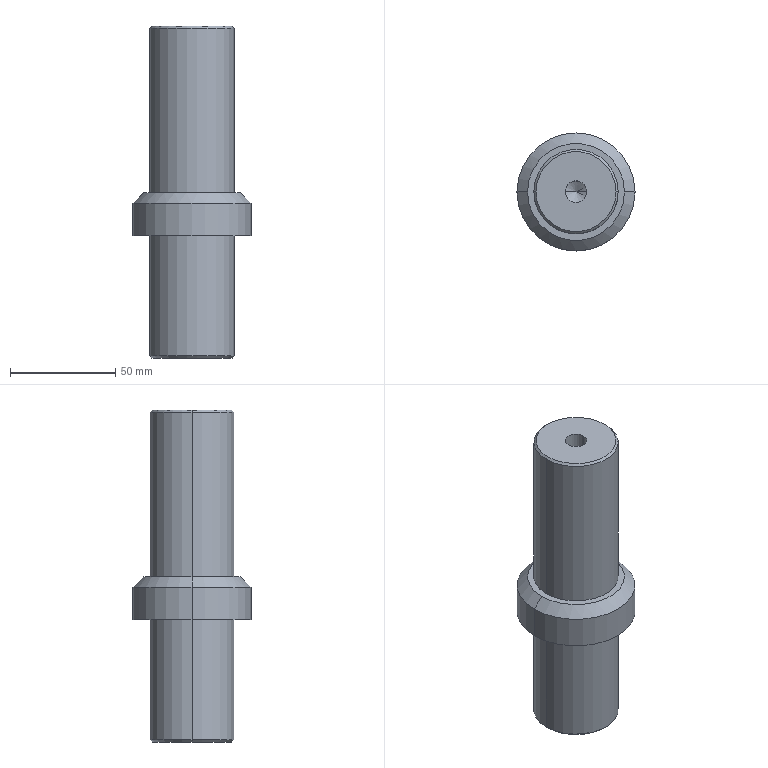Part | SolidWorks | features Chamfer 2, HoleWzd 2, ICE 2, Extrusion 1 | 1 solid | 24 faces | box 56 x 56 x 157.5 mm | volume 215391 mm3 | cylinder 10 | cone 10 | plane 4 | commonest cylinder face diameters 10.2 x4 40 x4 56 x2
STEP:
#1=CARTESIAN_POINT('',(-5.1,0.,128.25));
#2=VERTEX_POINT('',#1);
#3=CARTESIAN_POINT('',(5.1,0.,128.25));
#4=VERTEX_POINT('',#3);
#5=CARTESIAN_POINT('',(0.,0.,128.25));
#6=DIRECTION('',(0.,0.,1.));
#7=DIRECTION('',(1.,0.,0.));
#8=AXIS2_PLACEMENT_3D('',#5,#6,#7);
#9=CIRCLE('',#8,5.1);
#10=EDGE_CURVE('',#2,#4,#9,.T.);
#11=ORIENTED_EDGE('',*,*,#10,.F.);
#12=CARTESIAN_POINT('',(-5.1,0.,157.5));
#13=VERTEX_POINT('',#12);
#14=CARTESIAN_POINT('',(-5.1,0.,157.5));
#15=DIRECTION('',(0.,0.,1.));
#16=VECTOR('',#15,1000.);
#17=LINE('',#14,#16);
#18=EDGE_CURVE('',#2,#13,#17,.T.);
#19=ORIENTED_EDGE('',*,*,#18,.T.);
#20=CARTESIAN_POINT('',(5.1,0.,157.5));
#21=VERTEX_POINT('',#20);
#22=CARTESIAN_POINT('',(0.,0.,157.5));
#23=DIRECTION('',(0.,0.,1.));
#24=DIRECTION('',(1.,0.,0.));
#25=AXIS2_PLACEMENT_3D('',#22,#23,#24);
#26=CIRCLE('',#25,5.1);
#27=EDGE_CURVE('',#13,#21,#26,.T.);
#28=ORIENTED_EDGE('',*,*,#27,.T.);
#29=CARTESIAN_POINT('',(5.1,0.,157.5));
#30=DIRECTION('',(0.,0.,1.));
#31=VECTOR('',#30,1000.);
#32=LINE('',#29,#31);
#33=EDGE_CURVE('',#4,#21,#32,.T.);
#34=ORIENTED_EDGE('',*,*,#33,.F.);
#35=EDGE_LOOP('',(#11,#19,#28,#34));
#36=FACE_OUTER_BOUND('',#35,.T.);
#37=CARTESIAN_POINT('',(0.,0.,157.5));
#38=DIRECTION('',(0.,0.,1.));
#39=DIRECTION('',(1.,0.,0.));
#40=AXIS2_PLACEMENT_3D('',#37,#38,#39);
#41=CYLINDRICAL_SURFACE('',#40,5.1);
#42=ADVANCED_FACE('',(#36),#41,.F.);
#43=CARTESIAN_POINT('',(0.,0.,125.186));
#44=VERTEX_POINT('',#43);
#45=CARTESIAN_POINT('',(5.1,0.,128.25));
#46=DIRECTION('',(0.8572,0.,0.515));
#47=VECTOR('',#46,1000.);
#48=LINE('',#45,#47);
#49=EDGE_CURVE('',#44,#4,#48,.T.);
#50=ORIENTED_EDGE('',*,*,#49,.F.);
#51=CARTESIAN_POINT('',(-5.1,0.,128.25));
#52=DIRECTION('',(-0.8572,0.,0.515));
#53=VECTOR('',#52,1000.);
#54=LINE('',#51,#53);
#55=EDGE_CURVE('',#44,#2,#54,.T.);
#56=ORIENTED_EDGE('',*,*,#55,.T.);
#57=ORIENTED_EDGE('',*,*,#10,.T.);
#58=EDGE_LOOP('',(#50,#56,#57));
#59=FACE_OUTER_BOUND('',#58,.T.);
#60=CARTESIAN_POINT('',(0.,0.,128.25));
#61=DIRECTION('',(0.,0.,1.));
#62=DIRECTION('',(1.,0.,0.));
#63=AXIS2_PLACEMENT_3D('',#60,#61,#62);
#64=CONICAL_SURFACE('',#63,5.1,1.03);
#65=ADVANCED_FACE('',(#59),#64,.F.);
#66=CARTESIAN_POINT('',(5.1,0.,29.25));
#67=VERTEX_POINT('',#66);
#68=CARTESIAN_POINT('',(-5.1,0.,29.25));
#69=VERTEX_POINT('',#68);
#70=CARTESIAN_POINT('',(0.,0.,29.25));
#71=DIRECTION('',(0.,0.,-1.));
#72=DIRECTION('',(-1.,0.,0.));
#73=AXIS2_PLACEMENT_3D('',#70,#71,#72);
#74=CIRCLE('',#73,5.1);
#75=EDGE_CURVE('',#67,#69,#74,.T.);
#76=ORIENTED_EDGE('',*,*,#75,.F.);
#77=CARTESIAN_POINT('',(5.1,0.,0.));
#78=VERTEX_POINT('',#77);
#79=CARTESIAN_POINT('',(5.1,0.,0.));
#80=DIRECTION('',(0.,0.,-1.));
#81=VECTOR('',#80,1000.);
#82=LINE('',#79,#81);
#83=EDGE_CURVE('',#67,#78,#82,.T.);
#84=ORIENTED_EDGE('',*,*,#83,.T.);
#85=CARTESIAN_POINT('',(-5.1,0.,0.));
#86=VERTEX_POINT('',#85);
#87=CARTESIAN_POINT('',(0.,0.,0.));
#88=DIRECTION('',(0.,0.,-1.));
#89=DIRECTION('',(-1.,0.,0.));
#90=AXIS2_PLACEMENT_3D('',#87,#88,#89);
#91=CIRCLE('',#90,5.1);
#92=EDGE_CURVE('',#78,#86,#91,.T.);
#93=ORIENTED_EDGE('',*,*,#92,.T.);
#94=CARTESIAN_POINT('',(-5.1,0.,0.));
#95=DIRECTION('',(0.,0.,-1.));
#96=VECTOR('',#95,1000.);
#97=LINE('',#94,#96);
#98=EDGE_CURVE('',#69,#86,#97,.T.);
#99=ORIENTED_EDGE('',*,*,#98,.F.);
#100=EDGE_LOOP('',(#76,#84,#93,#99));
#101=FACE_OUTER_BOUND('',#100,.T.);
#102=CARTESIAN_POINT('',(0.,0.,0.));
#103=DIRECTION('',(0.,0.,-1.));
#104=DIRECTION('',(-1.,0.,0.));
#105=AXIS2_PLACEMENT_3D('',#102,#103,#104);
#106=CYLINDRICAL_SURFACE('',#105,5.1);
#107=ADVANCED_FACE('',(#101),#106,.F.);
#108=CARTESIAN_POINT('',(0.,0.,32.314));
#109=VERTEX_POINT('',#108);
#110=CARTESIAN_POINT('',(-5.1,0.,29.25));
#111=DIRECTION('',(-0.8572,0.,-0.515));
#112=VECTOR('',#111,1000.);
#113=LINE('',#110,#112);
#114=EDGE_CURVE('',#109,#69,#113,.T.);
#115=ORIENTED_EDGE('',*,*,#114,.F.);
#116=CARTESIAN_POINT('',(5.1,0.,29.25));
#117=DIRECTION('',(0.8572,0.,-0.515));
#118=VECTOR('',#117,1000.);
#119=LINE('',#116,#118);
#120=EDGE_CURVE('',#109,#67,#119,.T.);
#121=ORIENTED_EDGE('',*,*,#120,.T.);
#122=ORIENTED_EDGE('',*,*,#75,.T.);
#123=EDGE_LOOP('',(#115,#121,#122));
#124=FACE_OUTER_BOUND('',#123,.T.);
#125=CARTESIAN_POINT('',(0.,0.,29.25));
#126=DIRECTION('',(0.,0.,-1.));
#127=DIRECTION('',(-1.,0.,0.));
#128=AXIS2_PLACEMENT_3D('',#125,#126,#127);
#129=CONICAL_SURFACE('',#128,5.1,1.03);
#130=ADVANCED_FACE('',(#124),#129,.F.);
#131=CARTESIAN_POINT('',(-19.,0.,0.));
#132=VERTEX_POINT('',#131);
#133=CARTESIAN_POINT('',(19.,0.,0.));
#134=VERTEX_POINT('',#133);
#135=CARTESIAN_POINT('',(0.,0.,0.));
#136=DIRECTION('',(0.,0.,-1.));
#137=DIRECTION('',(1.,0.,0.));
#138=AXIS2_PLACEMENT_3D('',#135,#136,#137);
#139=CIRCLE('',#138,19.);
#140=EDGE_CURVE('',#132,#134,#139,.T.);
#141=ORIENTED_EDGE('',*,*,#140,.F.);
#142=CARTESIAN_POINT('',(-20.,0.,1.));
#143=VERTEX_POINT('',#142);
#144=CARTESIAN_POINT('',(-20.,0.,1.));
#145=DIRECTION('',(-0.7071,0.,0.7071));
#146=VECTOR('',#145,1000.);
#147=LINE('',#144,#146);
#148=EDGE_CURVE('',#132,#143,#147,.T.);
#149=ORIENTED_EDGE('',*,*,#148,.T.);
#150=CARTESIAN_POINT('',(20.,0.,1.));
#151=VERTEX_POINT('',#150);
#152=CARTESIAN_POINT('',(0.,0.,1.));
#153=DIRECTION('',(0.,0.,1.));
#154=DIRECTION('',(1.,0.,0.));
#155=AXIS2_PLACEMENT_3D('',#152,#153,#154);
#156=CIRCLE('',#155,20.);
#157=EDGE_CURVE('',#151,#143,#156,.T.);
#158=ORIENTED_EDGE('',*,*,#157,.F.);
#159=CARTESIAN_POINT('',(20.,0.,1.));
#160=DIRECTION('',(0.7071,0.,0.7071));
#161=VECTOR('',#160,1000.);
#162=LINE('',#159,#161);
#163=EDGE_CURVE('',#134,#151,#162,.T.);
#164=ORIENTED_EDGE('',*,*,#163,.F.);
#165=EDGE_LOOP('',(#141,#149,#158,#164));
#166=FACE_OUTER_BOUND('',#165,.T.);
#167=CARTESIAN_POINT('',(0.,0.,1.));
#168=DIRECTION('',(0.,0.,1.));
#169=DIRECTION('',(1.,0.,0.));
#170=AXIS2_PLACEMENT_3D('',#167,#168,#169);
#171=CONICAL_SURFACE('',#170,20.,0.7854);
#172=ADVANCED_FACE('',(#166),#171,.T.);
#173=CARTESIAN_POINT('',(19.,0.,157.5));
#174=VERTEX_POINT('',#173);
#175=CARTESIAN_POINT('',(-19.,0.,157.5));
#176=VERTEX_POINT('',#175);
#177=CARTESIAN_POINT('',(0.,0.,157.5));
#178=DIRECTION('',(0.,0.,1.));
#179=DIRECTION('',(1.,0.,0.));
#180=AXIS2_PLACEMENT_3D('',#177,#178,#179);
#181=CIRCLE('',#180,19.);
#182=EDGE_CURVE('',#174,#176,#181,.T.);
#183=ORIENTED_EDGE('',*,*,#182,.F.);
#184=CARTESIAN_POINT('',(20.,0.,156.5));
#185=VERTEX_POINT('',#184);
#186=CARTESIAN_POINT('',(19.,0.,157.5));
#187=DIRECTION('',(0.7071,0.,-0.7071));
#188=VECTOR('',#187,1000.);
#189=LINE('',#186,#188);
#190=EDGE_CURVE('',#174,#185,#189,.T.);
#191=ORIENTED_EDGE('',*,*,#190,.T.);
#192=CARTESIAN_POINT('',(-20.,0.,156.5));
#193=VERTEX_POINT('',#192);
#194=CARTESIAN_POINT('',(0.,0.,156.5));
#195=DIRECTION('',(0.,0.,-1.));
#196=DIRECTION('',(1.,0.,0.));
#197=AXIS2_PLACEMENT_3D('',#194,#195,#196);
#198=CIRCLE('',#197,20.);
#199=EDGE_CURVE('',#193,#185,#198,.T.);
#200=ORIENTED_EDGE('',*,*,#199,.F.);
#201=CARTESIAN_POINT('',(-19.,0.,157.5));
#202=DIRECTION('',(-0.7071,0.,-0.7071));
#203=VECTOR('',#202,1000.);
#204=LINE('',#201,#203);
#205=EDGE_CURVE('',#176,#193,#204,.T.);
#206=ORIENTED_EDGE('',*,*,#205,.F.);
#207=EDGE_LOOP('',(#183,#191,#200,#206));
#208=FACE_OUTER_BOUND('',#207,.T.);
#209=CARTESIAN_POINT('',(0.,0.,157.5));
#210=DIRECTION('',(0.,0.,-1.));
#211=DIRECTION('',(-1.,0.,0.));
#212=AXIS2_PLACEMENT_3D('',#209,#210,#211);
#213=CONICAL_SURFACE('',#212,19.,0.7854);
#214=ADVANCED_FACE('',(#208),#213,.T.);
#215=CARTESIAN_POINT('',(23.,0.,78.4));
#216=VERTEX_POINT('',#215);
#217=CARTESIAN_POINT('',(-23.,0.,78.4));
#218=VERTEX_POINT('',#217);
#219=CARTESIAN_POINT('',(0.,0.,78.4));
#220=DIRECTION('',(0.,0.,1.));
#221=DIRECTION('',(1.,0.,0.));
#222=AXIS2_PLACEMENT_3D('',#219,#220,#221);
#223=CIRCLE('',#222,23.);
#224=EDGE_CURVE('',#216,#218,#223,.T.);
#225=ORIENTED_EDGE('',*,*,#224,.F.);
#226=CARTESIAN_POINT('',(28.,0.,73.4));
#227=VERTEX_POINT('',#226);
#228=CARTESIAN_POINT('',(23.,0.,78.4));
#229=DIRECTION('',(0.7071,0.,-0.7071));
#230=VECTOR('',#229,1000.);
#231=LINE('',#228,#230);
#232=EDGE_CURVE('',#216,#227,#231,.T.);
#233=ORIENTED_EDGE('',*,*,#232,.T.);
#234=CARTESIAN_POINT('',(-28.,0.,73.4));
#235=VERTEX_POINT('',#234);
#236=CARTESIAN_POINT('',(0.,0.,73.4));
#237=DIRECTION('',(0.,0.,-1.));
#238=DIRECTION('',(1.,0.,0.));
#239=AXIS2_PLACEMENT_3D('',#236,#237,#238);
#240=CIRCLE('',#239,28.);
#241=EDGE_CURVE('',#235,#227,#240,.T.);
#242=ORIENTED_EDGE('',*,*,#241,.F.);
#243=CARTESIAN_POINT('',(-23.,0.,78.4));
#244=DIRECTION('',(-0.7071,0.,-0.7071));
#245=VECTOR('',#244,1000.);
#246=LINE('',#243,#245);
#247=EDGE_CURVE('',#218,#235,#246,.T.);
#248=ORIENTED_EDGE('',*,*,#247,.F.);
#249=EDGE_LOOP('',(#225,#233,#242,#248));
#250=FACE_OUTER_BOUND('',#249,.T.);
#251=CARTESIAN_POINT('',(0.,0.,78.4));
#252=DIRECTION('',(0.,0.,-1.));
#253=DIRECTION('',(-1.,0.,0.));
#254=AXIS2_PLACEMENT_3D('',#251,#252,#253);
#255=CONICAL_SURFACE('',#254,23.,0.7854);
#256=ADVANCED_FACE('',(#250),#255,.T.);
#257=ORIENTED_EDGE('',*,*,#199,.T.);
#258=CARTESIAN_POINT('',(20.,0.,78.4));
#259=VERTEX_POINT('',#258);
#260=CARTESIAN_POINT('',(20.,0.,157.5));
#261=DIRECTION('',(0.,0.,-1.));
#262=VECTOR('',#261,1000.);
#263=LINE('',#260,#262);
#264=EDGE_CURVE('',#185,#259,#263,.T.);
#265=ORIENTED_EDGE('',*,*,#264,.T.);
#266=CARTESIAN_POINT('',(-20.,0.,78.4));
#267=VERTEX_POINT('',#266);
#268=CARTESIAN_POINT('',(0.,0.,78.4));
#269=DIRECTION('',(0.,0.,1.));
#270=DIRECTION('',(1.,0.,0.));
#271=AXIS2_PLACEMENT_3D('',#268,#269,#270);
#272=CIRCLE('',#271,20.);
#273=EDGE_CURVE('',#259,#267,#272,.T.);
#274=ORIENTED_EDGE('',*,*,#273,.T.);
#275=CARTESIAN_POINT('',(-20.,0.,157.5));
#276=DIRECTION('',(0.,0.,-1.));
#277=VECTOR('',#276,1000.);
#278=LINE('',#275,#277);
#279=EDGE_CURVE('',#193,#267,#278,.T.);
#280=ORIENTED_EDGE('',*,*,#279,.F.);
#281=EDGE_LOOP('',(#257,#265,#274,#280));
#282=FACE_OUTER_BOUND('',#281,.T.);
#283=CARTESIAN_POINT('',(0.,0.,157.5));
#284=DIRECTION('',(0.,0.,-1.));
#285=DIRECTION('',(-1.,0.,0.));
#286=AXIS2_PLACEMENT_3D('',#283,#284,#285);
#287=CYLINDRICAL_SURFACE('',#286,20.);
#288=ADVANCED_FACE('',(#282),#287,.T.);
#289=ORIENTED_EDGE('',*,*,#241,.T.);
#290=CARTESIAN_POINT('',(28.,0.,58.));
#291=VERTEX_POINT('',#290);
#292=CARTESIAN_POINT('',(28.,0.,78.4));
#293=DIRECTION('',(0.,0.,-1.));
#294=VECTOR('',#293,1000.);
#295=LINE('',#292,#294);
#296=EDGE_CURVE('',#227,#291,#295,.T.);
#297=ORIENTED_EDGE('',*,*,#296,.T.);
#298=CARTESIAN_POINT('',(-28.,0.,58.));
#299=VERTEX_POINT('',#298);
#300=CARTESIAN_POINT('',(0.,0.,58.));
#301=DIRECTION('',(0.,0.,1.));
#302=DIRECTION('',(1.,0.,0.));
#303=AXIS2_PLACEMENT_3D('',#300,#301,#302);
#304=CIRCLE('',#303,28.);
#305=EDGE_CURVE('',#291,#299,#304,.T.);
#306=ORIENTED_EDGE('',*,*,#305,.T.);
#307=CARTESIAN_POINT('',(-28.,0.,78.4));
#308=DIRECTION('',(0.,0.,-1.));
#309=VECTOR('',#308,1000.);
#310=LINE('',#307,#309);
#311=EDGE_CURVE('',#235,#299,#310,.T.);
#312=ORIENTED_EDGE('',*,*,#311,.F.);
#313=EDGE_LOOP('',(#289,#297,#306,#312));
#314=FACE_OUTER_BOUND('',#313,.T.);
#315=CARTESIAN_POINT('',(0.,0.,78.4));
#316=DIRECTION('',(0.,0.,-1.));
#317=DIRECTION('',(-1.,0.,0.));
#318=AXIS2_PLACEMENT_3D('',#315,#316,#317);
#319=CYLINDRICAL_SURFACE('',#318,28.);
#320=ADVANCED_FACE('',(#314),#319,.T.);
#321=CARTESIAN_POINT('',(20.,0.,58.));
#322=VERTEX_POINT('',#321);
#323=CARTESIAN_POINT('',(-20.,0.,58.));
#324=VERTEX_POINT('',#323);
#325=CARTESIAN_POINT('',(0.,0.,58.));
#326=DIRECTION('',(0.,0.,1.));
#327=DIRECTION('',(1.,0.,0.));
#328=AXIS2_PLACEMENT_3D('',#325,#326,#327);
#329=CIRCLE('',#328,20.);
#330=EDGE_CURVE('',#322,#324,#329,.T.);
#331=ORIENTED_EDGE('',*,*,#330,.F.);
#332=CARTESIAN_POINT('',(20.,0.,58.));
#333=DIRECTION('',(0.,0.,-1.));
#334=VECTOR('',#333,1000.);
#335=LINE('',#332,#334);
#336=EDGE_CURVE('',#322,#151,#335,.T.);
#337=ORIENTED_EDGE('',*,*,#336,.T.);
#338=ORIENTED_EDGE('',*,*,#157,.T.);
#339=CARTESIAN_POINT('',(-20.,0.,58.));
#340=DIRECTION('',(0.,0.,-1.));
#341=VECTOR('',#340,1000.);
#342=LINE('',#339,#341);
#343=EDGE_CURVE('',#324,#143,#342,.T.);
#344=ORIENTED_EDGE('',*,*,#343,.F.);
#345=EDGE_LOOP('',(#331,#337,#338,#344));
#346=FACE_OUTER_BOUND('',#345,.T.);
#347=CARTESIAN_POINT('',(0.,0.,58.));
#348=DIRECTION('',(0.,0.,-1.));
#349=DIRECTION('',(-1.,0.,0.));
#350=AXIS2_PLACEMENT_3D('',#347,#348,#349);
#351=CYLINDRICAL_SURFACE('',#350,20.);
#352=ADVANCED_FACE('',(#346),#351,.T.);
#353=ORIENTED_EDGE('',*,*,#336,.F.);
#354=CARTESIAN_POINT('',(0.,0.,58.));
#355=DIRECTION('',(0.,0.,1.));
#356=DIRECTION('',(1.,0.,0.));
#357=AXIS2_PLACEMENT_3D('',#354,#355,#356);
#358=CIRCLE('',#357,20.);
#359=EDGE_CURVE('',#324,#322,#358,.T.);
#360=ORIENTED_EDGE('',*,*,#359,.F.);
#361=ORIENTED_EDGE('',*,*,#343,.T.);
#362=CARTESIAN_POINT('',(0.,0.,1.));
#363=DIRECTION('',(0.,0.,1.));
#364=DIRECTION('',(1.,0.,0.));
#365=AXIS2_PLACEMENT_3D('',#362,#363,#364);
#366=CIRCLE('',#365,20.);
#367=EDGE_CURVE('',#143,#151,#366,.T.);
#368=ORIENTED_EDGE('',*,*,#367,.T.);
#369=EDGE_LOOP('',(#353,#360,#361,#368));
#370=FACE_OUTER_BOUND('',#369,.T.);
#371=CARTESIAN_POINT('',(0.,0.,58.));
#372=DIRECTION('',(0.,0.,-1.));
#373=DIRECTION('',(-1.,0.,0.));
#374=AXIS2_PLACEMENT_3D('',#371,#372,#373);
#375=CYLINDRICAL_SURFACE('',#374,20.);
#376=ADVANCED_FACE('',(#370),#375,.T.);
#377=CARTESIAN_POINT('',(0.,0.,0.));
#378=DIRECTION('',(0.,0.,-1.));
#379=DIRECTION('',(-1.,0.,0.));
#380=AXIS2_PLACEMENT_3D('',#377,#378,#379);
#381=CIRCLE('',#380,5.1);
#382=EDGE_CURVE('',#86,#78,#381,.T.);
#383=ORIENTED_EDGE('',*,*,#382,.F.);
#384=ORIENTED_EDGE('',*,*,#92,.F.);
#385=EDGE_LOOP('',(#383,#384));
#386=FACE_BOUND('',#385,.T.);
#387=CARTESIAN_POINT('',(0.,0.,0.));
#388=DIRECTION('',(0.,0.,-1.));
#389=DIRECTION('',(1.,0.,0.));
#390=AXIS2_PLACEMENT_3D('',#387,#388,#389);
#391=CIRCLE('',#390,19.);
#392=EDGE_CURVE('',#134,#132,#391,.T.);
#393=ORIENTED_EDGE('',*,*,#392,.T.);
#394=ORIENTED_EDGE('',*,*,#140,.T.);
#395=EDGE_LOOP('',(#393,#394));
#396=FACE_OUTER_BOUND('',#395,.T.);
#397=CARTESIAN_POINT('',(0.,0.,0.));
#398=DIRECTION('',(0.,0.,1.));
#399=DIRECTION('',(1.,0.,0.));
#400=AXIS2_PLACEMENT_3D('',#397,#398,#399);
#401=PLANE('',#400);
#402=ADVANCED_FACE('',(#386,#396),#401,.F.);
#403=ORIENTED_EDGE('',*,*,#296,.F.);
#404=CARTESIAN_POINT('',(0.,0.,73.4));
#405=DIRECTION('',(0.,0.,-1.));
#406=DIRECTION('',(1.,0.,0.));
#407=AXIS2_PLACEMENT_3D('',#404,#405,#406);
#408=CIRCLE('',#407,28.);
#409=EDGE_CURVE('',#227,#235,#408,.T.);
#410=ORIENTED_EDGE('',*,*,#409,.T.);
#411=ORIENTED_EDGE('',*,*,#311,.T.);
#412=CARTESIAN_POINT('',(0.,0.,58.));
#413=DIRECTION('',(0.,0.,1.));
#414=DIRECTION('',(1.,0.,0.));
#415=AXIS2_PLACEMENT_3D('',#412,#413,#414);
#416=CIRCLE('',#415,28.);
#417=EDGE_CURVE('',#299,#291,#416,.T.);
#418=ORIENTED_EDGE('',*,*,#417,.T.);
#419=EDGE_LOOP('',(#403,#410,#411,#418));
#420=FACE_OUTER_BOUND('',#419,.T.);
#421=CARTESIAN_POINT('',(0.,0.,78.4));
#422=DIRECTION('',(0.,0.,-1.));
#423=DIRECTION('',(-1.,0.,0.));
#424=AXIS2_PLACEMENT_3D('',#421,#422,#423);
#425=CYLINDRICAL_SURFACE('',#424,28.);
#426=ADVANCED_FACE('',(#420),#425,.T.);
#427=CARTESIAN_POINT('',(0.,0.,78.4));
#428=DIRECTION('',(0.,0.,1.));
#429=DIRECTION('',(1.,0.,0.));
#430=AXIS2_PLACEMENT_3D('',#427,#428,#429);
#431=CIRCLE('',#430,23.);
#432=EDGE_CURVE('',#218,#216,#431,.T.);
#433=ORIENTED_EDGE('',*,*,#432,.T.);
#434=ORIENTED_EDGE('',*,*,#224,.T.);
#435=EDGE_LOOP('',(#433,#434));
#436=FACE_OUTER_BOUND('',#435,.T.);
#437=CARTESIAN_POINT('',(0.,0.,78.4));
#438=DIRECTION('',(0.,0.,1.));
#439=DIRECTION('',(1.,0.,0.));
#440=AXIS2_PLACEMENT_3D('',#437,#438,#439);
#441=CIRCLE('',#440,20.);
#442=EDGE_CURVE('',#267,#259,#441,.T.);
#443=ORIENTED_EDGE('',*,*,#442,.F.);
#444=ORIENTED_EDGE('',*,*,#273,.F.);
#445=EDGE_LOOP('',(#443,#444));
#446=FACE_BOUND('',#445,.T.);
#447=CARTESIAN_POINT('',(0.,0.,78.4));
#448=DIRECTION('',(0.,0.,1.));
#449=DIRECTION('',(1.,0.,0.));
#450=AXIS2_PLACEMENT_3D('',#447,#448,#449);
#451=PLANE('',#450);
#452=ADVANCED_FACE('',(#436,#446),#451,.T.);
#453=ORIENTED_EDGE('',*,*,#359,.T.);
#454=ORIENTED_EDGE('',*,*,#330,.T.);
#455=EDGE_LOOP('',(#453,#454));
#456=FACE_BOUND('',#455,.T.);
#457=ORIENTED_EDGE('',*,*,#417,.F.);
#458=ORIENTED_EDGE('',*,*,#305,.F.);
#459=EDGE_LOOP('',(#457,#458));
#460=FACE_OUTER_BOUND('',#459,.T.);
#461=CARTESIAN_POINT('',(0.,0.,58.));
#462=DIRECTION('',(0.,0.,1.));
#463=DIRECTION('',(1.,0.,0.));
#464=AXIS2_PLACEMENT_3D('',#461,#462,#463);
#465=PLANE('',#464);
#466=ADVANCED_FACE('',(#456,#460),#465,.F.);
#467=ORIENTED_EDGE('',*,*,#264,.F.);
#468=CARTESIAN_POINT('',(0.,0.,156.5));
#469=DIRECTION('',(0.,0.,-1.));
#470=DIRECTION('',(1.,0.,0.));
#471=AXIS2_PLACEMENT_3D('',#468,#469,#470);
#472=CIRCLE('',#471,20.);
#473=EDGE_CURVE('',#185,#193,#472,.T.);
#474=ORIENTED_EDGE('',*,*,#473,.T.);
#475=ORIENTED_EDGE('',*,*,#279,.T.);
#476=ORIENTED_EDGE('',*,*,#442,.T.);
#477=EDGE_LOOP('',(#467,#474,#475,#476));
#478=FACE_OUTER_BOUND('',#477,.T.);
#479=CARTESIAN_POINT('',(0.,0.,157.5));
#480=DIRECTION('',(0.,0.,-1.));
#481=DIRECTION('',(-1.,0.,0.));
#482=AXIS2_PLACEMENT_3D('',#479,#480,#481);
#483=CYLINDRICAL_SURFACE('',#482,20.);
#484=ADVANCED_FACE('',(#478),#483,.T.);
#485=CARTESIAN_POINT('',(0.,0.,157.5));
#486=DIRECTION('',(0.,0.,1.));
#487=DIRECTION('',(1.,0.,0.));
#488=AXIS2_PLACEMENT_3D('',#485,#486,#487);
#489=CIRCLE('',#488,5.1);
#490=EDGE_CURVE('',#21,#13,#489,.T.);
#491=ORIENTED_EDGE('',*,*,#490,.F.);
#492=ORIENTED_EDGE('',*,*,#27,.F.);
#493=EDGE_LOOP('',(#491,#492));
#494=FACE_BOUND('',#493,.T.);
#495=CARTESIAN_POINT('',(0.,0.,157.5));
#496=DIRECTION('',(0.,0.,1.));
#497=DIRECTION('',(1.,0.,0.));
#498=AXIS2_PLACEMENT_3D('',#495,#496,#497);
#499=CIRCLE('',#498,19.);
#500=EDGE_CURVE('',#176,#174,#499,.T.);
#501=ORIENTED_EDGE('',*,*,#500,.T.);
#502=ORIENTED_EDGE('',*,*,#182,.T.);
#503=EDGE_LOOP('',(#501,#502));
#504=FACE_OUTER_BOUND('',#503,.T.);
#505=CARTESIAN_POINT('',(0.,0.,157.5));
#506=DIRECTION('',(0.,0.,1.));
#507=DIRECTION('',(1.,0.,0.));
#508=AXIS2_PLACEMENT_3D('',#505,#506,#507);
#509=PLANE('',#508);
#510=ADVANCED_FACE('',(#494,#504),#509,.T.);
#511=ORIENTED_EDGE('',*,*,#232,.F.);
#512=ORIENTED_EDGE('',*,*,#432,.F.);
#513=ORIENTED_EDGE('',*,*,#247,.T.);
#514=ORIENTED_EDGE('',*,*,#409,.F.);
#515=EDGE_LOOP('',(#511,#512,#513,#514));
#516=FACE_OUTER_BOUND('',#515,.T.);
#517=CARTESIAN_POINT('',(0.,0.,78.4));
#518=DIRECTION('',(0.,0.,-1.));
#519=DIRECTION('',(-1.,0.,0.));
#520=AXIS2_PLACEMENT_3D('',#517,#518,#519);
#521=CONICAL_SURFACE('',#520,23.,0.7854);
#522=ADVANCED_FACE('',(#516),#521,.T.);
#523=ORIENTED_EDGE('',*,*,#190,.F.);
#524=ORIENTED_EDGE('',*,*,#500,.F.);
#525=ORIENTED_EDGE('',*,*,#205,.T.);
#526=ORIENTED_EDGE('',*,*,#473,.F.);
#527=EDGE_LOOP('',(#523,#524,#525,#526));
#528=FACE_OUTER_BOUND('',#527,.T.);
#529=CARTESIAN_POINT('',(0.,0.,157.5));
#530=DIRECTION('',(0.,0.,-1.));
#531=DIRECTION('',(-1.,0.,0.));
#532=AXIS2_PLACEMENT_3D('',#529,#530,#531);
#533=CONICAL_SURFACE('',#532,19.,0.7854);
#534=ADVANCED_FACE('',(#528),#533,.T.);
#535=ORIENTED_EDGE('',*,*,#148,.F.);
#536=ORIENTED_EDGE('',*,*,#392,.F.);
#537=ORIENTED_EDGE('',*,*,#163,.T.);
#538=ORIENTED_EDGE('',*,*,#367,.F.);
#539=EDGE_LOOP('',(#535,#536,#537,#538));
#540=FACE_OUTER_BOUND('',#539,.T.);
#541=CARTESIAN_POINT('',(0.,0.,1.));
#542=DIRECTION('',(0.,0.,1.));
#543=DIRECTION('',(1.,0.,0.));
#544=AXIS2_PLACEMENT_3D('',#541,#542,#543);
#545=CONICAL_SURFACE('',#544,20.,0.7854);
#546=ADVANCED_FACE('',(#540),#545,.T.);
#547=ORIENTED_EDGE('',*,*,#120,.F.);
#548=ORIENTED_EDGE('',*,*,#114,.T.);
#549=CARTESIAN_POINT('',(0.,0.,29.25));
#550=DIRECTION('',(0.,0.,-1.));
#551=DIRECTION('',(-1.,0.,0.));
#552=AXIS2_PLACEMENT_3D('',#549,#550,#551);
#553=CIRCLE('',#552,5.1);
#554=EDGE_CURVE('',#69,#67,#553,.T.);
#555=ORIENTED_EDGE('',*,*,#554,.T.);
#556=EDGE_LOOP('',(#547,#548,#555));
#557=FACE_OUTER_BOUND('',#556,.T.);
#558=CARTESIAN_POINT('',(0.,0.,29.25));
#559=DIRECTION('',(0.,0.,-1.));
#560=DIRECTION('',(-1.,0.,0.));
#561=AXIS2_PLACEMENT_3D('',#558,#559,#560);
#562=CONICAL_SURFACE('',#561,5.1,1.03);
#563=ADVANCED_FACE('',(#557),#562,.F.);
#564=ORIENTED_EDGE('',*,*,#83,.F.);
#565=ORIENTED_EDGE('',*,*,#554,.F.);
#566=ORIENTED_EDGE('',*,*,#98,.T.);
#567=ORIENTED_EDGE('',*,*,#382,.T.);
#568=EDGE_LOOP('',(#564,#565,#566,#567));
#569=FACE_OUTER_BOUND('',#568,.T.);
#570=CARTESIAN_POINT('',(0.,0.,0.));
#571=DIRECTION('',(0.,0.,-1.));
#572=DIRECTION('',(-1.,0.,0.));
#573=AXIS2_PLACEMENT_3D('',#570,#571,#572);
#574=CYLINDRICAL_SURFACE('',#573,5.1);
#575=ADVANCED_FACE('',(#569),#574,.F.);
#576=ORIENTED_EDGE('',*,*,#55,.F.);
#577=ORIENTED_EDGE('',*,*,#49,.T.);
#578=CARTESIAN_POINT('',(0.,0.,128.25));
#579=DIRECTION('',(0.,0.,1.));
#580=DIRECTION('',(1.,0.,0.));
#581=AXIS2_PLACEMENT_3D('',#578,#579,#580);
#582=CIRCLE('',#581,5.1);
#583=EDGE_CURVE('',#4,#2,#582,.T.);
#584=ORIENTED_EDGE('',*,*,#583,.T.);
#585=EDGE_LOOP('',(#576,#577,#584));
#586=FACE_OUTER_BOUND('',#585,.T.);
#587=CARTESIAN_POINT('',(0.,0.,128.25));
#588=DIRECTION('',(0.,0.,1.));
#589=DIRECTION('',(1.,0.,0.));
#590=AXIS2_PLACEMENT_3D('',#587,#588,#589);
#591=CONICAL_SURFACE('',#590,5.1,1.03);
#592=ADVANCED_FACE('',(#586),#591,.F.);
#593=ORIENTED_EDGE('',*,*,#18,.F.);
#594=ORIENTED_EDGE('',*,*,#583,.F.);
#595=ORIENTED_EDGE('',*,*,#33,.T.);
#596=ORIENTED_EDGE('',*,*,#490,.T.);
#597=EDGE_LOOP('',(#593,#594,#595,#596));
#598=FACE_OUTER_BOUND('',#597,.T.);
#599=CARTESIAN_POINT('',(0.,0.,157.5));
#600=DIRECTION('',(0.,0.,1.));
#601=DIRECTION('',(1.,0.,0.));
#602=AXIS2_PLACEMENT_3D('',#599,#600,#601);
#603=CYLINDRICAL_SURFACE('',#602,5.1);
#604=ADVANCED_FACE('',(#598),#603,.F.);
#605=CLOSED_SHELL('',(#42,#65,#107,#130,#172,#214,#256,#288,#320,#352,#376,#402,#426,#452,#466,#484,#510,#522,#534,#546,#563,#575,#592,#604));
#606=MANIFOLD_SOLID_BREP('',#605);
#607=CARTESIAN_POINT('',(0.,0.,0.));
#608=DIRECTION('',(0.,0.,1.));
#609=DIRECTION('',(1.,0.,0.));
#610=AXIS2_PLACEMENT_3D('',#607,#608,#609);
#611=(LENGTH_UNIT()NAMED_UNIT(*)SI_UNIT(.MILLI.,.METRE.));
#612=UNCERTAINTY_MEASURE_WITH_UNIT(LENGTH_MEASURE(0.00001),#611,'','');
#613=(NAMED_UNIT(*)PLANE_ANGLE_UNIT()SI_UNIT($,.RADIAN.));
#614=(NAMED_UNIT(*)SI_UNIT($,.STERADIAN.)SOLID_ANGLE_UNIT());
#615=(GEOMETRIC_REPRESENTATION_CONTEXT(3)GLOBAL_UNCERTAINTY_ASSIGNED_CONTEXT((#612))GLOBAL_UNIT_ASSIGNED_CONTEXT((#611,#613,#614))REPRESENTATION_CONTEXT('',''));
#616=ADVANCED_BREP_SHAPE_REPRESENTATION('',(#606,#610),#615);